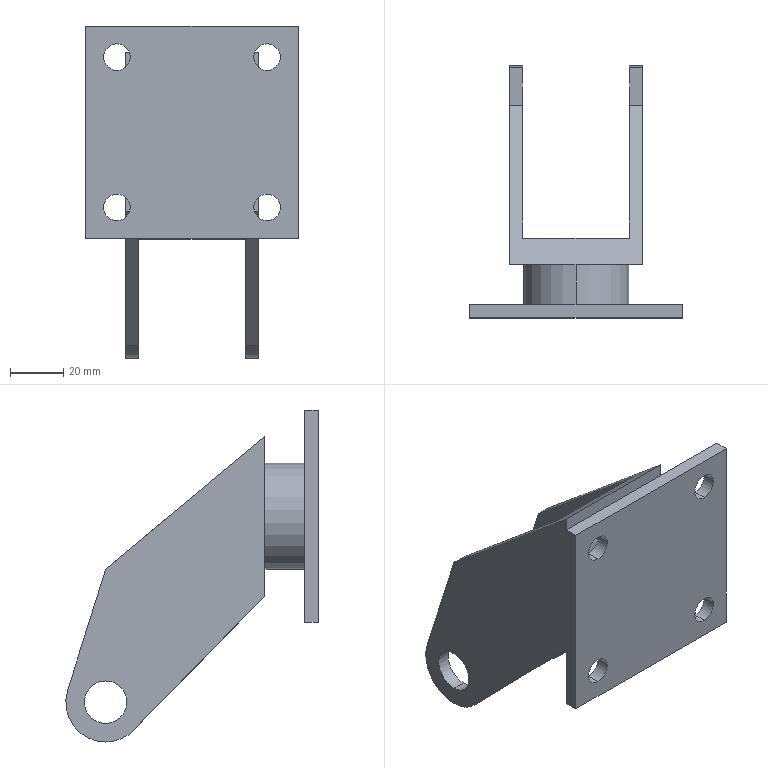Part | SolidWorks | features ICE 3, Extrusion 1 | 1 solid | 34 faces | box 80 x 95 x 125 mm | volume 116525 mm3 | cylinder 18 | plane 16 | commonest cylinder face diameters 10 x8 16 x4 30 x4 40 x2
STEP:
#1=CARTESIAN_POINT('',(0.,20.,20.));
#2=VERTEX_POINT('',#1);
#3=CARTESIAN_POINT('',(0.,20.,-20.));
#4=VERTEX_POINT('',#3);
#5=CARTESIAN_POINT('',(0.,20.,0.));
#6=DIRECTION('',(0.,1.,0.));
#7=DIRECTION('',(0.,0.,1.));
#8=AXIS2_PLACEMENT_3D('',#5,#6,#7);
#9=CIRCLE('',#8,20.);
#10=EDGE_CURVE('',#2,#4,#9,.T.);
#11=ORIENTED_EDGE('',*,*,#10,.F.);
#12=CARTESIAN_POINT('',(0.,5.,20.));
#13=VERTEX_POINT('',#12);
#14=CARTESIAN_POINT('',(0.,20.,20.));
#15=DIRECTION('',(0.,-1.,0.));
#16=VECTOR('',#15,1000.);
#17=LINE('',#14,#16);
#18=EDGE_CURVE('',#2,#13,#17,.T.);
#19=ORIENTED_EDGE('',*,*,#18,.T.);
#20=CARTESIAN_POINT('',(0.,5.,-20.));
#21=VERTEX_POINT('',#20);
#22=CARTESIAN_POINT('',(0.,5.,0.));
#23=DIRECTION('',(0.,1.,0.));
#24=DIRECTION('',(0.,0.,1.));
#25=AXIS2_PLACEMENT_3D('',#22,#23,#24);
#26=CIRCLE('',#25,20.);
#27=EDGE_CURVE('',#13,#21,#26,.T.);
#28=ORIENTED_EDGE('',*,*,#27,.T.);
#29=CARTESIAN_POINT('',(0.,20.,-20.));
#30=DIRECTION('',(0.,-1.,0.));
#31=VECTOR('',#30,1000.);
#32=LINE('',#29,#31);
#33=EDGE_CURVE('',#4,#21,#32,.T.);
#34=ORIENTED_EDGE('',*,*,#33,.F.);
#35=EDGE_LOOP('',(#11,#19,#28,#34));
#36=FACE_OUTER_BOUND('',#35,.T.);
#37=CARTESIAN_POINT('',(0.,20.,0.));
#38=DIRECTION('',(0.,-1.,0.));
#39=DIRECTION('',(0.,0.,-1.));
#40=AXIS2_PLACEMENT_3D('',#37,#38,#39);
#41=CYLINDRICAL_SURFACE('',#40,20.);
#42=ADVANCED_FACE('',(#36),#41,.T.);
#43=CARTESIAN_POINT('',(28.284,5.,23.284));
#44=VERTEX_POINT('',#43);
#45=CARTESIAN_POINT('',(28.284,5.,33.284));
#46=VERTEX_POINT('',#45);
#47=CARTESIAN_POINT('',(28.284,5.,28.284));
#48=DIRECTION('',(0.,1.,0.));
#49=DIRECTION('',(0.,0.,1.));
#50=AXIS2_PLACEMENT_3D('',#47,#48,#49);
#51=CIRCLE('',#50,5.);
#52=EDGE_CURVE('',#44,#46,#51,.T.);
#53=ORIENTED_EDGE('',*,*,#52,.T.);
#54=CARTESIAN_POINT('',(28.284,0.,33.284));
#55=VERTEX_POINT('',#54);
#56=CARTESIAN_POINT('',(28.284,5.,33.284));
#57=DIRECTION('',(0.,-1.,0.));
#58=VECTOR('',#57,1000.);
#59=LINE('',#56,#58);
#60=EDGE_CURVE('',#46,#55,#59,.T.);
#61=ORIENTED_EDGE('',*,*,#60,.T.);
#62=CARTESIAN_POINT('',(28.284,0.,23.284));
#63=VERTEX_POINT('',#62);
#64=CARTESIAN_POINT('',(28.284,0.,28.284));
#65=DIRECTION('',(0.,1.,0.));
#66=DIRECTION('',(0.,0.,1.));
#67=AXIS2_PLACEMENT_3D('',#64,#65,#66);
#68=CIRCLE('',#67,5.);
#69=EDGE_CURVE('',#63,#55,#68,.T.);
#70=ORIENTED_EDGE('',*,*,#69,.F.);
#71=CARTESIAN_POINT('',(28.284,5.,23.284));
#72=DIRECTION('',(0.,-1.,0.));
#73=VECTOR('',#72,1000.);
#74=LINE('',#71,#73);
#75=EDGE_CURVE('',#44,#63,#74,.T.);
#76=ORIENTED_EDGE('',*,*,#75,.F.);
#77=EDGE_LOOP('',(#53,#61,#70,#76));
#78=FACE_OUTER_BOUND('',#77,.T.);
#79=CARTESIAN_POINT('',(28.284,5.,28.284));
#80=DIRECTION('',(0.,-1.,0.));
#81=DIRECTION('',(0.,0.,-1.));
#82=AXIS2_PLACEMENT_3D('',#79,#80,#81);
#83=CYLINDRICAL_SURFACE('',#82,5.);
#84=ADVANCED_FACE('',(#78),#83,.F.);
#85=CARTESIAN_POINT('',(28.284,5.,-33.284));
#86=VERTEX_POINT('',#85);
#87=CARTESIAN_POINT('',(28.284,5.,-23.284));
#88=VERTEX_POINT('',#87);
#89=CARTESIAN_POINT('',(28.284,5.,-28.284));
#90=DIRECTION('',(0.,1.,0.));
#91=DIRECTION('',(0.,0.,1.));
#92=AXIS2_PLACEMENT_3D('',#89,#90,#91);
#93=CIRCLE('',#92,5.);
#94=EDGE_CURVE('',#86,#88,#93,.T.);
#95=ORIENTED_EDGE('',*,*,#94,.T.);
#96=CARTESIAN_POINT('',(28.284,0.,-23.284));
#97=VERTEX_POINT('',#96);
#98=CARTESIAN_POINT('',(28.284,5.,-23.284));
#99=DIRECTION('',(0.,-1.,0.));
#100=VECTOR('',#99,1000.);
#101=LINE('',#98,#100);
#102=EDGE_CURVE('',#88,#97,#101,.T.);
#103=ORIENTED_EDGE('',*,*,#102,.T.);
#104=CARTESIAN_POINT('',(28.284,0.,-33.284));
#105=VERTEX_POINT('',#104);
#106=CARTESIAN_POINT('',(28.284,0.,-28.284));
#107=DIRECTION('',(0.,1.,0.));
#108=DIRECTION('',(0.,0.,1.));
#109=AXIS2_PLACEMENT_3D('',#106,#107,#108);
#110=CIRCLE('',#109,5.);
#111=EDGE_CURVE('',#105,#97,#110,.T.);
#112=ORIENTED_EDGE('',*,*,#111,.F.);
#113=CARTESIAN_POINT('',(28.284,5.,-33.284));
#114=DIRECTION('',(0.,-1.,0.));
#115=VECTOR('',#114,1000.);
#116=LINE('',#113,#115);
#117=EDGE_CURVE('',#86,#105,#116,.T.);
#118=ORIENTED_EDGE('',*,*,#117,.F.);
#119=EDGE_LOOP('',(#95,#103,#112,#118));
#120=FACE_OUTER_BOUND('',#119,.T.);
#121=CARTESIAN_POINT('',(28.284,5.,-28.284));
#122=DIRECTION('',(0.,-1.,0.));
#123=DIRECTION('',(0.,0.,-1.));
#124=AXIS2_PLACEMENT_3D('',#121,#122,#123);
#125=CYLINDRICAL_SURFACE('',#124,5.);
#126=ADVANCED_FACE('',(#120),#125,.F.);
#127=CARTESIAN_POINT('',(-28.284,5.,-33.284));
#128=VERTEX_POINT('',#127);
#129=CARTESIAN_POINT('',(-28.284,5.,-23.284));
#130=VERTEX_POINT('',#129);
#131=CARTESIAN_POINT('',(-28.284,5.,-28.284));
#132=DIRECTION('',(0.,1.,0.));
#133=DIRECTION('',(0.,0.,1.));
#134=AXIS2_PLACEMENT_3D('',#131,#132,#133);
#135=CIRCLE('',#134,5.);
#136=EDGE_CURVE('',#128,#130,#135,.T.);
#137=ORIENTED_EDGE('',*,*,#136,.T.);
#138=CARTESIAN_POINT('',(-28.284,0.,-23.284));
#139=VERTEX_POINT('',#138);
#140=CARTESIAN_POINT('',(-28.284,5.,-23.284));
#141=DIRECTION('',(0.,-1.,0.));
#142=VECTOR('',#141,1000.);
#143=LINE('',#140,#142);
#144=EDGE_CURVE('',#130,#139,#143,.T.);
#145=ORIENTED_EDGE('',*,*,#144,.T.);
#146=CARTESIAN_POINT('',(-28.284,0.,-33.284));
#147=VERTEX_POINT('',#146);
#148=CARTESIAN_POINT('',(-28.284,0.,-28.284));
#149=DIRECTION('',(0.,1.,0.));
#150=DIRECTION('',(0.,0.,1.));
#151=AXIS2_PLACEMENT_3D('',#148,#149,#150);
#152=CIRCLE('',#151,5.);
#153=EDGE_CURVE('',#147,#139,#152,.T.);
#154=ORIENTED_EDGE('',*,*,#153,.F.);
#155=CARTESIAN_POINT('',(-28.284,5.,-33.284));
#156=DIRECTION('',(0.,-1.,0.));
#157=VECTOR('',#156,1000.);
#158=LINE('',#155,#157);
#159=EDGE_CURVE('',#128,#147,#158,.T.);
#160=ORIENTED_EDGE('',*,*,#159,.F.);
#161=EDGE_LOOP('',(#137,#145,#154,#160));
#162=FACE_OUTER_BOUND('',#161,.T.);
#163=CARTESIAN_POINT('',(-28.284,5.,-28.284));
#164=DIRECTION('',(0.,-1.,0.));
#165=DIRECTION('',(0.,0.,-1.));
#166=AXIS2_PLACEMENT_3D('',#163,#164,#165);
#167=CYLINDRICAL_SURFACE('',#166,5.);
#168=ADVANCED_FACE('',(#162),#167,.F.);
#169=CARTESIAN_POINT('',(-28.284,5.,23.284));
#170=VERTEX_POINT('',#169);
#171=CARTESIAN_POINT('',(-28.284,5.,33.284));
#172=VERTEX_POINT('',#171);
#173=CARTESIAN_POINT('',(-28.284,5.,28.284));
#174=DIRECTION('',(0.,1.,0.));
#175=DIRECTION('',(0.,0.,1.));
#176=AXIS2_PLACEMENT_3D('',#173,#174,#175);
#177=CIRCLE('',#176,5.);
#178=EDGE_CURVE('',#170,#172,#177,.T.);
#179=ORIENTED_EDGE('',*,*,#178,.T.);
#180=CARTESIAN_POINT('',(-28.284,0.,33.284));
#181=VERTEX_POINT('',#180);
#182=CARTESIAN_POINT('',(-28.284,5.,33.284));
#183=DIRECTION('',(0.,-1.,0.));
#184=VECTOR('',#183,1000.);
#185=LINE('',#182,#184);
#186=EDGE_CURVE('',#172,#181,#185,.T.);
#187=ORIENTED_EDGE('',*,*,#186,.T.);
#188=CARTESIAN_POINT('',(-28.284,0.,23.284));
#189=VERTEX_POINT('',#188);
#190=CARTESIAN_POINT('',(-28.284,0.,28.284));
#191=DIRECTION('',(0.,1.,0.));
#192=DIRECTION('',(0.,0.,1.));
#193=AXIS2_PLACEMENT_3D('',#190,#191,#192);
#194=CIRCLE('',#193,5.);
#195=EDGE_CURVE('',#189,#181,#194,.T.);
#196=ORIENTED_EDGE('',*,*,#195,.F.);
#197=CARTESIAN_POINT('',(-28.284,5.,23.284));
#198=DIRECTION('',(0.,-1.,0.));
#199=VECTOR('',#198,1000.);
#200=LINE('',#197,#199);
#201=EDGE_CURVE('',#170,#189,#200,.T.);
#202=ORIENTED_EDGE('',*,*,#201,.F.);
#203=EDGE_LOOP('',(#179,#187,#196,#202));
#204=FACE_OUTER_BOUND('',#203,.T.);
#205=CARTESIAN_POINT('',(-28.284,5.,28.284));
#206=DIRECTION('',(0.,-1.,0.));
#207=DIRECTION('',(0.,0.,-1.));
#208=AXIS2_PLACEMENT_3D('',#205,#206,#207);
#209=CYLINDRICAL_SURFACE('',#208,5.);
#210=ADVANCED_FACE('',(#204),#209,.F.);
#211=CARTESIAN_POINT('',(20.,80.,-62.));
#212=VERTEX_POINT('',#211);
#213=CARTESIAN_POINT('',(20.,80.,-78.));
#214=VERTEX_POINT('',#213);
#215=CARTESIAN_POINT('',(20.,80.,-70.));
#216=DIRECTION('',(1.,0.,0.));
#217=DIRECTION('',(0.,0.,1.));
#218=AXIS2_PLACEMENT_3D('',#215,#216,#217);
#219=CIRCLE('',#218,8.);
#220=EDGE_CURVE('',#212,#214,#219,.T.);
#221=ORIENTED_EDGE('',*,*,#220,.F.);
#222=CARTESIAN_POINT('',(25.,80.,-62.));
#223=VERTEX_POINT('',#222);
#224=CARTESIAN_POINT('',(-25.,80.,-62.));
#225=DIRECTION('',(1.,0.,0.));
#226=VECTOR('',#225,1000.);
#227=LINE('',#224,#226);
#228=EDGE_CURVE('',#212,#223,#227,.T.);
#229=ORIENTED_EDGE('',*,*,#228,.T.);
#230=CARTESIAN_POINT('',(25.,80.,-78.));
#231=VERTEX_POINT('',#230);
#232=CARTESIAN_POINT('',(25.,80.,-70.));
#233=DIRECTION('',(1.,0.,0.));
#234=DIRECTION('',(0.,0.,-1.));
#235=AXIS2_PLACEMENT_3D('',#232,#233,#234);
#236=CIRCLE('',#235,8.);
#237=EDGE_CURVE('',#223,#231,#236,.T.);
#238=ORIENTED_EDGE('',*,*,#237,.T.);
#239=CARTESIAN_POINT('',(-25.,80.,-78.));
#240=DIRECTION('',(1.,0.,0.));
#241=VECTOR('',#240,1000.);
#242=LINE('',#239,#241);
#243=EDGE_CURVE('',#214,#231,#242,.T.);
#244=ORIENTED_EDGE('',*,*,#243,.F.);
#245=EDGE_LOOP('',(#221,#229,#238,#244));
#246=FACE_OUTER_BOUND('',#245,.T.);
#247=CARTESIAN_POINT('',(-25.,80.,-70.));
#248=DIRECTION('',(1.,0.,0.));
#249=DIRECTION('',(0.,0.,-1.));
#250=AXIS2_PLACEMENT_3D('',#247,#248,#249);
#251=CYLINDRICAL_SURFACE('',#250,8.);
#252=ADVANCED_FACE('',(#246),#251,.F.);
#253=CARTESIAN_POINT('',(-25.,80.,-62.));
#254=VERTEX_POINT('',#253);
#255=CARTESIAN_POINT('',(-25.,80.,-78.));
#256=VERTEX_POINT('',#255);
#257=CARTESIAN_POINT('',(-25.,80.,-70.));
#258=DIRECTION('',(1.,0.,0.));
#259=DIRECTION('',(0.,0.,-1.));
#260=AXIS2_PLACEMENT_3D('',#257,#258,#259);
#261=CIRCLE('',#260,8.);
#262=EDGE_CURVE('',#254,#256,#261,.T.);
#263=ORIENTED_EDGE('',*,*,#262,.F.);
#264=CARTESIAN_POINT('',(-20.,80.,-62.));
#265=VERTEX_POINT('',#264);
#266=CARTESIAN_POINT('',(-25.,80.,-62.));
#267=DIRECTION('',(1.,0.,0.));
#268=VECTOR('',#267,1000.);
#269=LINE('',#266,#268);
#270=EDGE_CURVE('',#254,#265,#269,.T.);
#271=ORIENTED_EDGE('',*,*,#270,.T.);
#272=CARTESIAN_POINT('',(-20.,80.,-78.));
#273=VERTEX_POINT('',#272);
#274=CARTESIAN_POINT('',(-20.,80.,-70.));
#275=DIRECTION('',(-1.,0.,0.));
#276=DIRECTION('',(0.,0.,-1.));
#277=AXIS2_PLACEMENT_3D('',#274,#275,#276);
#278=CIRCLE('',#277,8.);
#279=EDGE_CURVE('',#273,#265,#278,.T.);
#280=ORIENTED_EDGE('',*,*,#279,.F.);
#281=CARTESIAN_POINT('',(-25.,80.,-78.));
#282=DIRECTION('',(1.,0.,0.));
#283=VECTOR('',#282,1000.);
#284=LINE('',#281,#283);
#285=EDGE_CURVE('',#256,#273,#284,.T.);
#286=ORIENTED_EDGE('',*,*,#285,.F.);
#287=EDGE_LOOP('',(#263,#271,#280,#286));
#288=FACE_OUTER_BOUND('',#287,.T.);
#289=CARTESIAN_POINT('',(-25.,80.,-70.));
#290=DIRECTION('',(1.,0.,0.));
#291=DIRECTION('',(0.,0.,-1.));
#292=AXIS2_PLACEMENT_3D('',#289,#290,#291);
#293=CYLINDRICAL_SURFACE('',#292,8.);
#294=ADVANCED_FACE('',(#288),#293,.F.);
#295=CARTESIAN_POINT('',(20.,69.265,-80.477));
#296=VERTEX_POINT('',#295);
#297=CARTESIAN_POINT('',(20.,80.,-85.));
#298=VERTEX_POINT('',#297);
#299=CARTESIAN_POINT('',(20.,80.,-70.));
#300=DIRECTION('',(1.,0.,0.));
#301=DIRECTION('',(0.,0.,1.));
#302=AXIS2_PLACEMENT_3D('',#299,#300,#301);
#303=CIRCLE('',#302,15.);
#304=EDGE_CURVE('',#296,#298,#303,.T.);
#305=ORIENTED_EDGE('',*,*,#304,.T.);
#306=CARTESIAN_POINT('',(25.,80.,-85.));
#307=VERTEX_POINT('',#306);
#308=CARTESIAN_POINT('',(-25.,80.,-85.));
#309=DIRECTION('',(1.,0.,0.));
#310=VECTOR('',#309,1000.);
#311=LINE('',#308,#310);
#312=EDGE_CURVE('',#298,#307,#311,.T.);
#313=ORIENTED_EDGE('',*,*,#312,.T.);
#314=CARTESIAN_POINT('',(25.,69.265,-80.477));
#315=VERTEX_POINT('',#314);
#316=CARTESIAN_POINT('',(25.,80.,-70.));
#317=DIRECTION('',(1.,0.,0.));
#318=DIRECTION('',(0.,0.,-1.));
#319=AXIS2_PLACEMENT_3D('',#316,#317,#318);
#320=CIRCLE('',#319,15.);
#321=EDGE_CURVE('',#315,#307,#320,.T.);
#322=ORIENTED_EDGE('',*,*,#321,.F.);
#323=CARTESIAN_POINT('',(-25.,69.265,-80.477));
#324=DIRECTION('',(1.,0.,0.));
#325=VECTOR('',#324,1000.);
#326=LINE('',#323,#325);
#327=EDGE_CURVE('',#296,#315,#326,.T.);
#328=ORIENTED_EDGE('',*,*,#327,.F.);
#329=EDGE_LOOP('',(#305,#313,#322,#328));
#330=FACE_OUTER_BOUND('',#329,.T.);
#331=CARTESIAN_POINT('',(-25.,80.,-70.));
#332=DIRECTION('',(1.,0.,0.));
#333=DIRECTION('',(0.,0.,-1.));
#334=AXIS2_PLACEMENT_3D('',#331,#332,#333);
#335=CYLINDRICAL_SURFACE('',#334,15.);
#336=ADVANCED_FACE('',(#330),#335,.T.);
#337=CARTESIAN_POINT('',(-25.,69.265,-80.477));
#338=VERTEX_POINT('',#337);
#339=CARTESIAN_POINT('',(-25.,80.,-85.));
#340=VERTEX_POINT('',#339);
#341=CARTESIAN_POINT('',(-25.,80.,-70.));
#342=DIRECTION('',(1.,0.,0.));
#343=DIRECTION('',(0.,0.,-1.));
#344=AXIS2_PLACEMENT_3D('',#341,#342,#343);
#345=CIRCLE('',#344,15.);
#346=EDGE_CURVE('',#338,#340,#345,.T.);
#347=ORIENTED_EDGE('',*,*,#346,.T.);
#348=CARTESIAN_POINT('',(-20.,80.,-85.));
#349=VERTEX_POINT('',#348);
#350=CARTESIAN_POINT('',(-25.,80.,-85.));
#351=DIRECTION('',(1.,0.,0.));
#352=VECTOR('',#351,1000.);
#353=LINE('',#350,#352);
#354=EDGE_CURVE('',#340,#349,#353,.T.);
#355=ORIENTED_EDGE('',*,*,#354,.T.);
#356=CARTESIAN_POINT('',(-20.,69.265,-80.477));
#357=VERTEX_POINT('',#356);
#358=CARTESIAN_POINT('',(-20.,80.,-70.));
#359=DIRECTION('',(-1.,0.,0.));
#360=DIRECTION('',(0.,0.,-1.));
#361=AXIS2_PLACEMENT_3D('',#358,#359,#360);
#362=CIRCLE('',#361,15.);
#363=EDGE_CURVE('',#349,#357,#362,.T.);
#364=ORIENTED_EDGE('',*,*,#363,.T.);
#365=CARTESIAN_POINT('',(-25.,69.265,-80.477));
#366=DIRECTION('',(1.,0.,0.));
#367=VECTOR('',#366,1000.);
#368=LINE('',#365,#367);
#369=EDGE_CURVE('',#338,#357,#368,.T.);
#370=ORIENTED_EDGE('',*,*,#369,.F.);
#371=EDGE_LOOP('',(#347,#355,#364,#370));
#372=FACE_OUTER_BOUND('',#371,.T.);
#373=CARTESIAN_POINT('',(-25.,80.,-70.));
#374=DIRECTION('',(1.,0.,0.));
#375=DIRECTION('',(0.,0.,-1.));
#376=AXIS2_PLACEMENT_3D('',#373,#374,#375);
#377=CYLINDRICAL_SURFACE('',#376,15.);
#378=ADVANCED_FACE('',(#372),#377,.T.);
#379=CARTESIAN_POINT('',(-20.,30.,21.667));
#380=VERTEX_POINT('',#379);
#381=CARTESIAN_POINT('',(20.,30.,21.667));
#382=VERTEX_POINT('',#381);
#383=CARTESIAN_POINT('',(-25.,30.,21.667));
#384=DIRECTION('',(1.,0.,0.));
#385=VECTOR('',#384,1000.);
#386=LINE('',#383,#385);
#387=EDGE_CURVE('',#380,#382,#386,.T.);
#388=ORIENTED_EDGE('',*,*,#387,.F.);
#389=CARTESIAN_POINT('',(-20.,80.,-20.));
#390=VERTEX_POINT('',#389);
#391=CARTESIAN_POINT('',(-20.,20.,30.));
#392=DIRECTION('',(0.,0.7682,-0.6402));
#393=VECTOR('',#392,1000.);
#394=LINE('',#391,#393);
#395=EDGE_CURVE('',#380,#390,#394,.T.);
#396=ORIENTED_EDGE('',*,*,#395,.T.);
#397=CARTESIAN_POINT('',(-25.,80.,-20.));
#398=VERTEX_POINT('',#397);
#399=CARTESIAN_POINT('',(-25.,80.,-20.));
#400=DIRECTION('',(1.,0.,0.));
#401=VECTOR('',#400,1000.);
#402=LINE('',#399,#401);
#403=EDGE_CURVE('',#398,#390,#402,.T.);
#404=ORIENTED_EDGE('',*,*,#403,.F.);
#405=CARTESIAN_POINT('',(-25.,20.,30.));
#406=VERTEX_POINT('',#405);
#407=CARTESIAN_POINT('',(-25.,20.,30.));
#408=DIRECTION('',(0.,-0.7682,0.6402));
#409=VECTOR('',#408,1000.);
#410=LINE('',#407,#409);
#411=EDGE_CURVE('',#398,#406,#410,.T.);
#412=ORIENTED_EDGE('',*,*,#411,.T.);
#413=CARTESIAN_POINT('',(25.,20.,30.));
#414=VERTEX_POINT('',#413);
#415=CARTESIAN_POINT('',(-25.,20.,30.));
#416=DIRECTION('',(1.,0.,0.));
#417=VECTOR('',#416,1000.);
#418=LINE('',#415,#417);
#419=EDGE_CURVE('',#406,#414,#418,.T.);
#420=ORIENTED_EDGE('',*,*,#419,.T.);
#421=CARTESIAN_POINT('',(25.,80.,-20.));
#422=VERTEX_POINT('',#421);
#423=CARTESIAN_POINT('',(25.,20.,30.));
#424=DIRECTION('',(0.,-0.7682,0.6402));
#425=VECTOR('',#424,1000.);
#426=LINE('',#423,#425);
#427=EDGE_CURVE('',#422,#414,#426,.T.);
#428=ORIENTED_EDGE('',*,*,#427,.F.);
#429=CARTESIAN_POINT('',(20.,80.,-20.));
#430=VERTEX_POINT('',#429);
#431=CARTESIAN_POINT('',(-25.,80.,-20.));
#432=DIRECTION('',(1.,0.,0.));
#433=VECTOR('',#432,1000.);
#434=LINE('',#431,#433);
#435=EDGE_CURVE('',#430,#422,#434,.T.);
#436=ORIENTED_EDGE('',*,*,#435,.F.);
#437=CARTESIAN_POINT('',(20.,20.,30.));
#438=DIRECTION('',(0.,-0.7682,0.6402));
#439=VECTOR('',#438,1000.);
#440=LINE('',#437,#439);
#441=EDGE_CURVE('',#430,#382,#440,.T.);
#442=ORIENTED_EDGE('',*,*,#441,.T.);
#443=EDGE_LOOP('',(#388,#396,#404,#412,#420,#428,#436,#442));
#444=FACE_OUTER_BOUND('',#443,.T.);
#445=CARTESIAN_POINT('',(-25.,20.,30.));
#446=DIRECTION('',(0.,0.6402,0.7682));
#447=DIRECTION('',(0.,-0.7682,0.6402));
#448=AXIS2_PLACEMENT_3D('',#445,#446,#447);
#449=PLANE('',#448);
#450=ADVANCED_FACE('',(#444),#449,.T.);
#451=ORIENTED_EDGE('',*,*,#403,.T.);
#452=CARTESIAN_POINT('',(-20.,94.309,-65.5));
#453=VERTEX_POINT('',#452);
#454=CARTESIAN_POINT('',(-20.,80.,-20.));
#455=DIRECTION('',(0.,0.3,-0.9539));
#456=VECTOR('',#455,1000.);
#457=LINE('',#454,#456);
#458=EDGE_CURVE('',#390,#453,#457,.T.);
#459=ORIENTED_EDGE('',*,*,#458,.T.);
#460=CARTESIAN_POINT('',(-25.,94.309,-65.5));
#461=VERTEX_POINT('',#460);
#462=CARTESIAN_POINT('',(-25.,94.309,-65.5));
#463=DIRECTION('',(1.,0.,0.));
#464=VECTOR('',#463,1000.);
#465=LINE('',#462,#464);
#466=EDGE_CURVE('',#461,#453,#465,.T.);
#467=ORIENTED_EDGE('',*,*,#466,.F.);
#468=CARTESIAN_POINT('',(-25.,80.,-20.));
#469=DIRECTION('',(0.,-0.3,0.9539));
#470=VECTOR('',#469,1000.);
#471=LINE('',#468,#470);
#472=EDGE_CURVE('',#461,#398,#471,.T.);
#473=ORIENTED_EDGE('',*,*,#472,.T.);
#474=EDGE_LOOP('',(#451,#459,#467,#473));
#475=FACE_OUTER_BOUND('',#474,.T.);
#476=CARTESIAN_POINT('',(-25.,80.,-20.));
#477=DIRECTION('',(0.,0.9539,0.3));
#478=DIRECTION('',(0.,-0.3,0.9539));
#479=AXIS2_PLACEMENT_3D('',#476,#477,#478);
#480=PLANE('',#479);
#481=ADVANCED_FACE('',(#475),#480,.T.);
#482=CARTESIAN_POINT('',(20.,94.309,-65.5));
#483=VERTEX_POINT('',#482);
#484=CARTESIAN_POINT('',(25.,94.309,-65.5));
#485=VERTEX_POINT('',#484);
#486=CARTESIAN_POINT('',(-25.,94.309,-65.5));
#487=DIRECTION('',(1.,0.,0.));
#488=VECTOR('',#487,1000.);
#489=LINE('',#486,#488);
#490=EDGE_CURVE('',#483,#485,#489,.T.);
#491=ORIENTED_EDGE('',*,*,#490,.F.);
#492=CARTESIAN_POINT('',(20.,80.,-20.));
#493=DIRECTION('',(0.,-0.3,0.9539));
#494=VECTOR('',#493,1000.);
#495=LINE('',#492,#494);
#496=EDGE_CURVE('',#483,#430,#495,.T.);
#497=ORIENTED_EDGE('',*,*,#496,.T.);
#498=ORIENTED_EDGE('',*,*,#435,.T.);
#499=CARTESIAN_POINT('',(25.,80.,-20.));
#500=DIRECTION('',(0.,-0.3,0.9539));
#501=VECTOR('',#500,1000.);
#502=LINE('',#499,#501);
#503=EDGE_CURVE('',#485,#422,#502,.T.);
#504=ORIENTED_EDGE('',*,*,#503,.F.);
#505=EDGE_LOOP('',(#491,#497,#498,#504));
#506=FACE_OUTER_BOUND('',#505,.T.);
#507=CARTESIAN_POINT('',(-25.,80.,-20.));
#508=DIRECTION('',(0.,0.9539,0.3));
#509=DIRECTION('',(0.,-0.3,0.9539));
#510=AXIS2_PLACEMENT_3D('',#507,#508,#509);
#511=PLANE('',#510);
#512=ADVANCED_FACE('',(#506),#511,.T.);
#513=ORIENTED_EDGE('',*,*,#354,.F.);
#514=CARTESIAN_POINT('',(-25.,80.,-70.));
#515=DIRECTION('',(1.,0.,0.));
#516=DIRECTION('',(0.,0.,-1.));
#517=AXIS2_PLACEMENT_3D('',#514,#515,#516);
#518=CIRCLE('',#517,15.);
#519=EDGE_CURVE('',#340,#461,#518,.T.);
#520=ORIENTED_EDGE('',*,*,#519,.T.);
#521=ORIENTED_EDGE('',*,*,#466,.T.);
#522=CARTESIAN_POINT('',(-20.,80.,-70.));
#523=DIRECTION('',(-1.,0.,0.));
#524=DIRECTION('',(0.,0.,-1.));
#525=AXIS2_PLACEMENT_3D('',#522,#523,#524);
#526=CIRCLE('',#525,15.);
#527=EDGE_CURVE('',#453,#349,#526,.T.);
#528=ORIENTED_EDGE('',*,*,#527,.T.);
#529=EDGE_LOOP('',(#513,#520,#521,#528));
#530=FACE_OUTER_BOUND('',#529,.T.);
#531=CARTESIAN_POINT('',(-25.,80.,-70.));
#532=DIRECTION('',(1.,0.,0.));
#533=DIRECTION('',(0.,0.,-1.));
#534=AXIS2_PLACEMENT_3D('',#531,#532,#533);
#535=CYLINDRICAL_SURFACE('',#534,15.);
#536=ADVANCED_FACE('',(#530),#535,.T.);
#537=ORIENTED_EDGE('',*,*,#312,.F.);
#538=CARTESIAN_POINT('',(20.,80.,-70.));
#539=DIRECTION('',(1.,0.,0.));
#540=DIRECTION('',(0.,0.,1.));
#541=AXIS2_PLACEMENT_3D('',#538,#539,#540);
#542=CIRCLE('',#541,15.);
#543=EDGE_CURVE('',#298,#483,#542,.T.);
#544=ORIENTED_EDGE('',*,*,#543,.T.);
#545=ORIENTED_EDGE('',*,*,#490,.T.);
#546=CARTESIAN_POINT('',(25.,80.,-70.));
#547=DIRECTION('',(1.,0.,0.));
#548=DIRECTION('',(0.,0.,-1.));
#549=AXIS2_PLACEMENT_3D('',#546,#547,#548);
#550=CIRCLE('',#549,15.);
#551=EDGE_CURVE('',#307,#485,#550,.T.);
#552=ORIENTED_EDGE('',*,*,#551,.F.);
#553=EDGE_LOOP('',(#537,#544,#545,#552));
#554=FACE_OUTER_BOUND('',#553,.T.);
#555=CARTESIAN_POINT('',(-25.,80.,-70.));
#556=DIRECTION('',(1.,0.,0.));
#557=DIRECTION('',(0.,0.,-1.));
#558=AXIS2_PLACEMENT_3D('',#555,#556,#557);
#559=CYLINDRICAL_SURFACE('',#558,15.);
#560=ADVANCED_FACE('',(#554),#559,.T.);
#561=ORIENTED_EDGE('',*,*,#369,.T.);
#562=CARTESIAN_POINT('',(-20.,30.,-40.246));
#563=VERTEX_POINT('',#562);
#564=CARTESIAN_POINT('',(-20.,20.,-30.));
#565=DIRECTION('',(0.,-0.6985,0.7156));
#566=VECTOR('',#565,1000.);
#567=LINE('',#564,#566);
#568=EDGE_CURVE('',#357,#563,#567,.T.);
#569=ORIENTED_EDGE('',*,*,#568,.T.);
#570=CARTESIAN_POINT('',(20.,30.,-40.246));
#571=VERTEX_POINT('',#570);
#572=CARTESIAN_POINT('',(-25.,30.,-40.246));
#573=DIRECTION('',(-1.,0.,0.));
#574=VECTOR('',#573,1000.);
#575=LINE('',#572,#574);
#576=EDGE_CURVE('',#571,#563,#575,.T.);
#577=ORIENTED_EDGE('',*,*,#576,.F.);
#578=CARTESIAN_POINT('',(20.,20.,-30.));
#579=DIRECTION('',(0.,0.6985,-0.7156));
#580=VECTOR('',#579,1000.);
#581=LINE('',#578,#580);
#582=EDGE_CURVE('',#571,#296,#581,.T.);
#583=ORIENTED_EDGE('',*,*,#582,.T.);
#584=ORIENTED_EDGE('',*,*,#327,.T.);
#585=CARTESIAN_POINT('',(25.,20.,-30.));
#586=VERTEX_POINT('',#585);
#587=CARTESIAN_POINT('',(25.,20.,-30.));
#588=DIRECTION('',(0.,0.6985,-0.7156));
#589=VECTOR('',#588,1000.);
#590=LINE('',#587,#589);
#591=EDGE_CURVE('',#586,#315,#590,.T.);
#592=ORIENTED_EDGE('',*,*,#591,.F.);
#593=CARTESIAN_POINT('',(-25.,20.,-30.));
#594=VERTEX_POINT('',#593);
#595=CARTESIAN_POINT('',(-25.,20.,-30.));
#596=DIRECTION('',(1.,0.,0.));
#597=VECTOR('',#596,1000.);
#598=LINE('',#595,#597);
#599=EDGE_CURVE('',#594,#586,#598,.T.);
#600=ORIENTED_EDGE('',*,*,#599,.F.);
#601=CARTESIAN_POINT('',(-25.,20.,-30.));
#602=DIRECTION('',(0.,0.6985,-0.7156));
#603=VECTOR('',#602,1000.);
#604=LINE('',#601,#603);
#605=EDGE_CURVE('',#594,#338,#604,.T.);
#606=ORIENTED_EDGE('',*,*,#605,.T.);
#607=EDGE_LOOP('',(#561,#569,#577,#583,#584,#592,#600,#606));
#608=FACE_OUTER_BOUND('',#607,.T.);
#609=CARTESIAN_POINT('',(-25.,20.,-30.));
#610=DIRECTION('',(0.,-0.7156,-0.6985));
#611=DIRECTION('',(0.,0.6985,-0.7156));
#612=AXIS2_PLACEMENT_3D('',#609,#610,#611);
#613=PLANE('',#612);
#614=ADVANCED_FACE('',(#608),#613,.T.);
#615=ORIENTED_EDGE('',*,*,#270,.F.);
#616=CARTESIAN_POINT('',(-25.,80.,-70.));
#617=DIRECTION('',(1.,0.,0.));
#618=DIRECTION('',(0.,0.,-1.));
#619=AXIS2_PLACEMENT_3D('',#616,#617,#618);
#620=CIRCLE('',#619,8.);
#621=EDGE_CURVE('',#256,#254,#620,.T.);
#622=ORIENTED_EDGE('',*,*,#621,.F.);
#623=ORIENTED_EDGE('',*,*,#285,.T.);
#624=CARTESIAN_POINT('',(-20.,80.,-70.));
#625=DIRECTION('',(-1.,0.,0.));
#626=DIRECTION('',(0.,0.,-1.));
#627=AXIS2_PLACEMENT_3D('',#624,#625,#626);
#628=CIRCLE('',#627,8.);
#629=EDGE_CURVE('',#265,#273,#628,.T.);
#630=ORIENTED_EDGE('',*,*,#629,.F.);
#631=EDGE_LOOP('',(#615,#622,#623,#630));
#632=FACE_OUTER_BOUND('',#631,.T.);
#633=CARTESIAN_POINT('',(-25.,80.,-70.));
#634=DIRECTION('',(1.,0.,0.));
#635=DIRECTION('',(0.,0.,-1.));
#636=AXIS2_PLACEMENT_3D('',#633,#634,#635);
#637=CYLINDRICAL_SURFACE('',#636,8.);
#638=ADVANCED_FACE('',(#632),#637,.F.);
#639=ORIENTED_EDGE('',*,*,#228,.F.);
#640=CARTESIAN_POINT('',(20.,80.,-70.));
#641=DIRECTION('',(1.,0.,0.));
#642=DIRECTION('',(0.,0.,1.));
#643=AXIS2_PLACEMENT_3D('',#640,#641,#642);
#644=CIRCLE('',#643,8.);
#645=EDGE_CURVE('',#214,#212,#644,.T.);
#646=ORIENTED_EDGE('',*,*,#645,.F.);
#647=ORIENTED_EDGE('',*,*,#243,.T.);
#648=CARTESIAN_POINT('',(25.,80.,-70.));
#649=DIRECTION('',(1.,0.,0.));
#650=DIRECTION('',(0.,0.,-1.));
#651=AXIS2_PLACEMENT_3D('',#648,#649,#650);
#652=CIRCLE('',#651,8.);
#653=EDGE_CURVE('',#231,#223,#652,.T.);
#654=ORIENTED_EDGE('',*,*,#653,.T.);
#655=EDGE_LOOP('',(#639,#646,#647,#654));
#656=FACE_OUTER_BOUND('',#655,.T.);
#657=CARTESIAN_POINT('',(-25.,80.,-70.));
#658=DIRECTION('',(1.,0.,0.));
#659=DIRECTION('',(0.,0.,-1.));
#660=AXIS2_PLACEMENT_3D('',#657,#658,#659);
#661=CYLINDRICAL_SURFACE('',#660,8.);
#662=ADVANCED_FACE('',(#656),#661,.F.);
#663=CARTESIAN_POINT('',(0.,5.,0.));
#664=DIRECTION('',(0.,1.,0.));
#665=DIRECTION('',(0.,0.,1.));
#666=AXIS2_PLACEMENT_3D('',#663,#664,#665);
#667=CIRCLE('',#666,20.);
#668=EDGE_CURVE('',#21,#13,#667,.T.);
#669=ORIENTED_EDGE('',*,*,#668,.F.);
#670=ORIENTED_EDGE('',*,*,#27,.F.);
#671=EDGE_LOOP('',(#669,#670));
#672=FACE_BOUND('',#671,.T.);
#673=ORIENTED_EDGE('',*,*,#94,.F.);
#674=CARTESIAN_POINT('',(28.284,5.,-28.284));
#675=DIRECTION('',(0.,1.,0.));
#676=DIRECTION('',(0.,0.,1.));
#677=AXIS2_PLACEMENT_3D('',#674,#675,#676);
#678=CIRCLE('',#677,5.);
#679=EDGE_CURVE('',#88,#86,#678,.T.);
#680=ORIENTED_EDGE('',*,*,#679,.F.);
#681=EDGE_LOOP('',(#673,#680));
#682=FACE_BOUND('',#681,.T.);
#683=ORIENTED_EDGE('',*,*,#178,.F.);
#684=CARTESIAN_POINT('',(-28.284,5.,28.284));
#685=DIRECTION('',(0.,1.,0.));
#686=DIRECTION('',(0.,0.,1.));
#687=AXIS2_PLACEMENT_3D('',#684,#685,#686);
#688=CIRCLE('',#687,5.);
#689=EDGE_CURVE('',#172,#170,#688,.T.);
#690=ORIENTED_EDGE('',*,*,#689,.F.);
#691=EDGE_LOOP('',(#683,#690));
#692=FACE_BOUND('',#691,.T.);
#693=CARTESIAN_POINT('',(40.,5.,40.));
#694=VERTEX_POINT('',#693);
#695=CARTESIAN_POINT('',(40.,5.,-40.));
#696=VERTEX_POINT('',#695);
#697=CARTESIAN_POINT('',(40.,5.,-40.));
#698=DIRECTION('',(0.,0.,-1.));
#699=VECTOR('',#698,1000.);
#700=LINE('',#697,#699);
#701=EDGE_CURVE('',#694,#696,#700,.T.);
#702=ORIENTED_EDGE('',*,*,#701,.T.);
#703=CARTESIAN_POINT('',(-40.,5.,-40.));
#704=VERTEX_POINT('',#703);
#705=CARTESIAN_POINT('',(-40.,5.,-40.));
#706=DIRECTION('',(-1.,0.,0.));
#707=VECTOR('',#706,1000.);
#708=LINE('',#705,#707);
#709=EDGE_CURVE('',#696,#704,#708,.T.);
#710=ORIENTED_EDGE('',*,*,#709,.T.);
#711=CARTESIAN_POINT('',(-40.,5.,40.));
#712=VERTEX_POINT('',#711);
#713=CARTESIAN_POINT('',(-40.,5.,-40.));
#714=DIRECTION('',(0.,0.,1.));
#715=VECTOR('',#714,1000.);
#716=LINE('',#713,#715);
#717=EDGE_CURVE('',#704,#712,#716,.T.);
#718=ORIENTED_EDGE('',*,*,#717,.T.);
#719=CARTESIAN_POINT('',(-40.,5.,40.));
#720=DIRECTION('',(1.,0.,0.));
#721=VECTOR('',#720,1000.);
#722=LINE('',#719,#721);
#723=EDGE_CURVE('',#712,#694,#722,.T.);
#724=ORIENTED_EDGE('',*,*,#723,.T.);
#725=EDGE_LOOP('',(#702,#710,#718,#724));
#726=FACE_OUTER_BOUND('',#725,.T.);
#727=ORIENTED_EDGE('',*,*,#136,.F.);
#728=CARTESIAN_POINT('',(-28.284,5.,-28.284));
#729=DIRECTION('',(0.,1.,0.));
#730=DIRECTION('',(0.,0.,1.));
#731=AXIS2_PLACEMENT_3D('',#728,#729,#730);
#732=CIRCLE('',#731,5.);
#733=EDGE_CURVE('',#130,#128,#732,.T.);
#734=ORIENTED_EDGE('',*,*,#733,.F.);
#735=EDGE_LOOP('',(#727,#734));
#736=FACE_BOUND('',#735,.T.);
#737=ORIENTED_EDGE('',*,*,#52,.F.);
#738=CARTESIAN_POINT('',(28.284,5.,28.284));
#739=DIRECTION('',(0.,1.,0.));
#740=DIRECTION('',(0.,0.,1.));
#741=AXIS2_PLACEMENT_3D('',#738,#739,#740);
#742=CIRCLE('',#741,5.);
#743=EDGE_CURVE('',#46,#44,#742,.T.);
#744=ORIENTED_EDGE('',*,*,#743,.F.);
#745=EDGE_LOOP('',(#737,#744));
#746=FACE_BOUND('',#745,.T.);
#747=CARTESIAN_POINT('',(0.,5.,0.));
#748=DIRECTION('',(0.,1.,0.));
#749=DIRECTION('',(0.,0.,1.));
#750=AXIS2_PLACEMENT_3D('',#747,#748,#749);
#751=PLANE('',#750);
#752=ADVANCED_FACE('',(#672,#682,#692,#726,#736,#746),#751,.T.);
#753=CARTESIAN_POINT('',(40.,0.,40.));
#754=VERTEX_POINT('',#753);
#755=CARTESIAN_POINT('',(40.,0.,-40.));
#756=VERTEX_POINT('',#755);
#757=CARTESIAN_POINT('',(40.,0.,-40.));
#758=DIRECTION('',(0.,0.,-1.));
#759=VECTOR('',#758,1000.);
#760=LINE('',#757,#759);
#761=EDGE_CURVE('',#754,#756,#760,.T.);
#762=ORIENTED_EDGE('',*,*,#761,.F.);
#763=CARTESIAN_POINT('',(-40.,0.,40.));
#764=VERTEX_POINT('',#763);
#765=CARTESIAN_POINT('',(-40.,0.,40.));
#766=DIRECTION('',(1.,0.,0.));
#767=VECTOR('',#766,1000.);
#768=LINE('',#765,#767);
#769=EDGE_CURVE('',#764,#754,#768,.T.);
#770=ORIENTED_EDGE('',*,*,#769,.F.);
#771=CARTESIAN_POINT('',(-40.,0.,-40.));
#772=VERTEX_POINT('',#771);
#773=CARTESIAN_POINT('',(-40.,0.,-40.));
#774=DIRECTION('',(0.,0.,1.));
#775=VECTOR('',#774,1000.);
#776=LINE('',#773,#775);
#777=EDGE_CURVE('',#772,#764,#776,.T.);
#778=ORIENTED_EDGE('',*,*,#777,.F.);
#779=CARTESIAN_POINT('',(-40.,0.,-40.));
#780=DIRECTION('',(-1.,0.,0.));
#781=VECTOR('',#780,1000.);
#782=LINE('',#779,#781);
#783=EDGE_CURVE('',#756,#772,#782,.T.);
#784=ORIENTED_EDGE('',*,*,#783,.F.);
#785=EDGE_LOOP('',(#762,#770,#778,#784));
#786=FACE_OUTER_BOUND('',#785,.T.);
#787=ORIENTED_EDGE('',*,*,#195,.T.);
#788=CARTESIAN_POINT('',(-28.284,0.,28.284));
#789=DIRECTION('',(0.,1.,0.));
#790=DIRECTION('',(0.,0.,1.));
#791=AXIS2_PLACEMENT_3D('',#788,#789,#790);
#792=CIRCLE('',#791,5.);
#793=EDGE_CURVE('',#181,#189,#792,.T.);
#794=ORIENTED_EDGE('',*,*,#793,.T.);
#795=EDGE_LOOP('',(#787,#794));
#796=FACE_BOUND('',#795,.T.);
#797=ORIENTED_EDGE('',*,*,#153,.T.);
#798=CARTESIAN_POINT('',(-28.284,0.,-28.284));
#799=DIRECTION('',(0.,1.,0.));
#800=DIRECTION('',(0.,0.,1.));
#801=AXIS2_PLACEMENT_3D('',#798,#799,#800);
#802=CIRCLE('',#801,5.);
#803=EDGE_CURVE('',#139,#147,#802,.T.);
#804=ORIENTED_EDGE('',*,*,#803,.T.);
#805=EDGE_LOOP('',(#797,#804));
#806=FACE_BOUND('',#805,.T.);
#807=ORIENTED_EDGE('',*,*,#111,.T.);
#808=CARTESIAN_POINT('',(28.284,0.,-28.284));
#809=DIRECTION('',(0.,1.,0.));
#810=DIRECTION('',(0.,0.,1.));
#811=AXIS2_PLACEMENT_3D('',#808,#809,#810);
#812=CIRCLE('',#811,5.);
#813=EDGE_CURVE('',#97,#105,#812,.T.);
#814=ORIENTED_EDGE('',*,*,#813,.T.);
#815=EDGE_LOOP('',(#807,#814));
#816=FACE_BOUND('',#815,.T.);
#817=ORIENTED_EDGE('',*,*,#69,.T.);
#818=CARTESIAN_POINT('',(28.284,0.,28.284));
#819=DIRECTION('',(0.,1.,0.));
#820=DIRECTION('',(0.,0.,1.));
#821=AXIS2_PLACEMENT_3D('',#818,#819,#820);
#822=CIRCLE('',#821,5.);
#823=EDGE_CURVE('',#55,#63,#822,.T.);
#824=ORIENTED_EDGE('',*,*,#823,.T.);
#825=EDGE_LOOP('',(#817,#824));
#826=FACE_BOUND('',#825,.T.);
#827=CARTESIAN_POINT('',(0.,0.,0.));
#828=DIRECTION('',(0.,1.,0.));
#829=DIRECTION('',(0.,0.,1.));
#830=AXIS2_PLACEMENT_3D('',#827,#828,#829);
#831=PLANE('',#830);
#832=ADVANCED_FACE('',(#786,#796,#806,#816,#826),#831,.F.);
#833=ORIENTED_EDGE('',*,*,#761,.T.);
#834=CARTESIAN_POINT('',(40.,5.,-40.));
#835=DIRECTION('',(0.,-1.,0.));
#836=VECTOR('',#835,1000.);
#837=LINE('',#834,#836);
#838=EDGE_CURVE('',#696,#756,#837,.T.);
#839=ORIENTED_EDGE('',*,*,#838,.F.);
#840=ORIENTED_EDGE('',*,*,#701,.F.);
#841=CARTESIAN_POINT('',(40.,5.,40.));
#842=DIRECTION('',(0.,-1.,0.));
#843=VECTOR('',#842,1000.);
#844=LINE('',#841,#843);
#845=EDGE_CURVE('',#694,#754,#844,.T.);
#846=ORIENTED_EDGE('',*,*,#845,.T.);
#847=EDGE_LOOP('',(#833,#839,#840,#846));
#848=FACE_OUTER_BOUND('',#847,.T.);
#849=CARTESIAN_POINT('',(40.,5.,-40.));
#850=DIRECTION('',(-1.,0.,0.));
#851=DIRECTION('',(0.,0.,1.));
#852=AXIS2_PLACEMENT_3D('',#849,#850,#851);
#853=PLANE('',#852);
#854=ADVANCED_FACE('',(#848),#853,.F.);
#855=ORIENTED_EDGE('',*,*,#783,.T.);
#856=CARTESIAN_POINT('',(-40.,5.,-40.));
#857=DIRECTION('',(0.,-1.,0.));
#858=VECTOR('',#857,1000.);
#859=LINE('',#856,#858);
#860=EDGE_CURVE('',#704,#772,#859,.T.);
#861=ORIENTED_EDGE('',*,*,#860,.F.);
#862=ORIENTED_EDGE('',*,*,#709,.F.);
#863=ORIENTED_EDGE('',*,*,#838,.T.);
#864=EDGE_LOOP('',(#855,#861,#862,#863));
#865=FACE_OUTER_BOUND('',#864,.T.);
#866=CARTESIAN_POINT('',(-40.,5.,-40.));
#867=DIRECTION('',(0.,0.,1.));
#868=DIRECTION('',(1.,0.,0.));
#869=AXIS2_PLACEMENT_3D('',#866,#867,#868);
#870=PLANE('',#869);
#871=ADVANCED_FACE('',(#865),#870,.F.);
#872=ORIENTED_EDGE('',*,*,#777,.T.);
#873=CARTESIAN_POINT('',(-40.,5.,40.));
#874=DIRECTION('',(0.,-1.,0.));
#875=VECTOR('',#874,1000.);
#876=LINE('',#873,#875);
#877=EDGE_CURVE('',#712,#764,#876,.T.);
#878=ORIENTED_EDGE('',*,*,#877,.F.);
#879=ORIENTED_EDGE('',*,*,#717,.F.);
#880=ORIENTED_EDGE('',*,*,#860,.T.);
#881=EDGE_LOOP('',(#872,#878,#879,#880));
#882=FACE_OUTER_BOUND('',#881,.T.);
#883=CARTESIAN_POINT('',(-40.,5.,-40.));
#884=DIRECTION('',(1.,0.,0.));
#885=DIRECTION('',(0.,0.,-1.));
#886=AXIS2_PLACEMENT_3D('',#883,#884,#885);
#887=PLANE('',#886);
#888=ADVANCED_FACE('',(#882),#887,.F.);
#889=ORIENTED_EDGE('',*,*,#769,.T.);
#890=ORIENTED_EDGE('',*,*,#845,.F.);
#891=ORIENTED_EDGE('',*,*,#723,.F.);
#892=ORIENTED_EDGE('',*,*,#877,.T.);
#893=EDGE_LOOP('',(#889,#890,#891,#892));
#894=FACE_OUTER_BOUND('',#893,.T.);
#895=CARTESIAN_POINT('',(-40.,5.,40.));
#896=DIRECTION('',(0.,0.,-1.));
#897=DIRECTION('',(-1.,0.,0.));
#898=AXIS2_PLACEMENT_3D('',#895,#896,#897);
#899=PLANE('',#898);
#900=ADVANCED_FACE('',(#894),#899,.F.);
#901=ORIENTED_EDGE('',*,*,#186,.F.);
#902=ORIENTED_EDGE('',*,*,#689,.T.);
#903=ORIENTED_EDGE('',*,*,#201,.T.);
#904=ORIENTED_EDGE('',*,*,#793,.F.);
#905=EDGE_LOOP('',(#901,#902,#903,#904));
#906=FACE_OUTER_BOUND('',#905,.T.);
#907=CARTESIAN_POINT('',(-28.284,5.,28.284));
#908=DIRECTION('',(0.,-1.,0.));
#909=DIRECTION('',(0.,0.,-1.));
#910=AXIS2_PLACEMENT_3D('',#907,#908,#909);
#911=CYLINDRICAL_SURFACE('',#910,5.);
#912=ADVANCED_FACE('',(#906),#911,.F.);
#913=ORIENTED_EDGE('',*,*,#144,.F.);
#914=ORIENTED_EDGE('',*,*,#733,.T.);
#915=ORIENTED_EDGE('',*,*,#159,.T.);
#916=ORIENTED_EDGE('',*,*,#803,.F.);
#917=EDGE_LOOP('',(#913,#914,#915,#916));
#918=FACE_OUTER_BOUND('',#917,.T.);
#919=CARTESIAN_POINT('',(-28.284,5.,-28.284));
#920=DIRECTION('',(0.,-1.,0.));
#921=DIRECTION('',(0.,0.,-1.));
#922=AXIS2_PLACEMENT_3D('',#919,#920,#921);
#923=CYLINDRICAL_SURFACE('',#922,5.);
#924=ADVANCED_FACE('',(#918),#923,.F.);
#925=ORIENTED_EDGE('',*,*,#102,.F.);
#926=ORIENTED_EDGE('',*,*,#679,.T.);
#927=ORIENTED_EDGE('',*,*,#117,.T.);
#928=ORIENTED_EDGE('',*,*,#813,.F.);
#929=EDGE_LOOP('',(#925,#926,#927,#928));
#930=FACE_OUTER_BOUND('',#929,.T.);
#931=CARTESIAN_POINT('',(28.284,5.,-28.284));
#932=DIRECTION('',(0.,-1.,0.));
#933=DIRECTION('',(0.,0.,-1.));
#934=AXIS2_PLACEMENT_3D('',#931,#932,#933);
#935=CYLINDRICAL_SURFACE('',#934,5.);
#936=ADVANCED_FACE('',(#930),#935,.F.);
#937=ORIENTED_EDGE('',*,*,#60,.F.);
#938=ORIENTED_EDGE('',*,*,#743,.T.);
#939=ORIENTED_EDGE('',*,*,#75,.T.);
#940=ORIENTED_EDGE('',*,*,#823,.F.);
#941=EDGE_LOOP('',(#937,#938,#939,#940));
#942=FACE_OUTER_BOUND('',#941,.T.);
#943=CARTESIAN_POINT('',(28.284,5.,28.284));
#944=DIRECTION('',(0.,-1.,0.));
#945=DIRECTION('',(0.,0.,-1.));
#946=AXIS2_PLACEMENT_3D('',#943,#944,#945);
#947=CYLINDRICAL_SURFACE('',#946,5.);
#948=ADVANCED_FACE('',(#942),#947,.F.);
#949=ORIENTED_EDGE('',*,*,#18,.F.);
#950=CARTESIAN_POINT('',(0.,20.,0.));
#951=DIRECTION('',(0.,1.,0.));
#952=DIRECTION('',(0.,0.,1.));
#953=AXIS2_PLACEMENT_3D('',#950,#951,#952);
#954=CIRCLE('',#953,20.);
#955=EDGE_CURVE('',#4,#2,#954,.T.);
#956=ORIENTED_EDGE('',*,*,#955,.F.);
#957=ORIENTED_EDGE('',*,*,#33,.T.);
#958=ORIENTED_EDGE('',*,*,#668,.T.);
#959=EDGE_LOOP('',(#949,#956,#957,#958));
#960=FACE_OUTER_BOUND('',#959,.T.);
#961=CARTESIAN_POINT('',(0.,20.,0.));
#962=DIRECTION('',(0.,-1.,0.));
#963=DIRECTION('',(0.,0.,-1.));
#964=AXIS2_PLACEMENT_3D('',#961,#962,#963);
#965=CYLINDRICAL_SURFACE('',#964,20.);
#966=ADVANCED_FACE('',(#960),#965,.T.);
#967=ORIENTED_EDGE('',*,*,#955,.T.);
#968=ORIENTED_EDGE('',*,*,#10,.T.);
#969=EDGE_LOOP('',(#967,#968));
#970=FACE_BOUND('',#969,.T.);
#971=ORIENTED_EDGE('',*,*,#599,.T.);
#972=CARTESIAN_POINT('',(25.,20.,0.));
#973=DIRECTION('',(0.,0.,-1.));
#974=VECTOR('',#973,1000.);
#975=LINE('',#972,#974);
#976=EDGE_CURVE('',#414,#586,#975,.T.);
#977=ORIENTED_EDGE('',*,*,#976,.F.);
#978=ORIENTED_EDGE('',*,*,#419,.F.);
#979=CARTESIAN_POINT('',(-25.,20.,0.));
#980=DIRECTION('',(0.,0.,-1.));
#981=VECTOR('',#980,1000.);
#982=LINE('',#979,#981);
#983=EDGE_CURVE('',#406,#594,#982,.T.);
#984=ORIENTED_EDGE('',*,*,#983,.T.);
#985=EDGE_LOOP('',(#971,#977,#978,#984));
#986=FACE_OUTER_BOUND('',#985,.T.);
#987=CARTESIAN_POINT('',(-25.,20.,0.));
#988=DIRECTION('',(0.,-1.,0.));
#989=DIRECTION('',(0.,0.,-1.));
#990=AXIS2_PLACEMENT_3D('',#987,#988,#989);
#991=PLANE('',#990);
#992=ADVANCED_FACE('',(#970,#986),#991,.T.);
#993=ORIENTED_EDGE('',*,*,#621,.T.);
#994=ORIENTED_EDGE('',*,*,#262,.T.);
#995=EDGE_LOOP('',(#993,#994));
#996=FACE_BOUND('',#995,.T.);
#997=ORIENTED_EDGE('',*,*,#983,.F.);
#998=ORIENTED_EDGE('',*,*,#411,.F.);
#999=ORIENTED_EDGE('',*,*,#472,.F.);
#1000=ORIENTED_EDGE('',*,*,#519,.F.);
#1001=ORIENTED_EDGE('',*,*,#346,.F.);
#1002=ORIENTED_EDGE('',*,*,#605,.F.);
#1003=EDGE_LOOP('',(#997,#998,#999,#1000,#1001,#1002));
#1004=FACE_OUTER_BOUND('',#1003,.T.);
#1005=CARTESIAN_POINT('',(-25.,80.,-70.));
#1006=DIRECTION('',(1.,0.,0.));
#1007=DIRECTION('',(0.,0.,-1.));
#1008=AXIS2_PLACEMENT_3D('',#1005,#1006,#1007);
#1009=PLANE('',#1008);
#1010=ADVANCED_FACE('',(#996,#1004),#1009,.F.);
#1011=ORIENTED_EDGE('',*,*,#976,.T.);
#1012=ORIENTED_EDGE('',*,*,#591,.T.);
#1013=ORIENTED_EDGE('',*,*,#321,.T.);
#1014=ORIENTED_EDGE('',*,*,#551,.T.);
#1015=ORIENTED_EDGE('',*,*,#503,.T.);
#1016=ORIENTED_EDGE('',*,*,#427,.T.);
#1017=EDGE_LOOP('',(#1011,#1012,#1013,#1014,#1015,#1016));
#1018=FACE_OUTER_BOUND('',#1017,.T.);
#1019=ORIENTED_EDGE('',*,*,#653,.F.);
#1020=ORIENTED_EDGE('',*,*,#237,.F.);
#1021=EDGE_LOOP('',(#1019,#1020));
#1022=FACE_BOUND('',#1021,.T.);
#1023=CARTESIAN_POINT('',(25.,80.,-70.));
#1024=DIRECTION('',(1.,0.,0.));
#1025=DIRECTION('',(0.,0.,-1.));
#1026=AXIS2_PLACEMENT_3D('',#1023,#1024,#1025);
#1027=PLANE('',#1026);
#1028=ADVANCED_FACE('',(#1018,#1022),#1027,.T.);
#1029=CARTESIAN_POINT('',(-20.,30.,-100.));
#1030=DIRECTION('',(0.,0.,-1.));
#1031=VECTOR('',#1030,1000.);
#1032=LINE('',#1029,#1031);
#1033=EDGE_CURVE('',#380,#563,#1032,.T.);
#1034=ORIENTED_EDGE('',*,*,#1033,.T.);
#1035=ORIENTED_EDGE('',*,*,#568,.F.);
#1036=ORIENTED_EDGE('',*,*,#363,.F.);
#1037=ORIENTED_EDGE('',*,*,#527,.F.);
#1038=ORIENTED_EDGE('',*,*,#458,.F.);
#1039=ORIENTED_EDGE('',*,*,#395,.F.);
#1040=EDGE_LOOP('',(#1034,#1035,#1036,#1037,#1038,#1039));
#1041=FACE_OUTER_BOUND('',#1040,.T.);
#1042=ORIENTED_EDGE('',*,*,#279,.T.);
#1043=ORIENTED_EDGE('',*,*,#629,.T.);
#1044=EDGE_LOOP('',(#1042,#1043));
#1045=FACE_BOUND('',#1044,.T.);
#1046=CARTESIAN_POINT('',(-20.,30.,-100.));
#1047=DIRECTION('',(1.,0.,0.));
#1048=DIRECTION('',(0.,0.,-1.));
#1049=AXIS2_PLACEMENT_3D('',#1046,#1047,#1048);
#1050=PLANE('',#1049);
#1051=ADVANCED_FACE('',(#1041,#1045),#1050,.T.);
#1052=ORIENTED_EDGE('',*,*,#496,.F.);
#1053=ORIENTED_EDGE('',*,*,#543,.F.);
#1054=ORIENTED_EDGE('',*,*,#304,.F.);
#1055=ORIENTED_EDGE('',*,*,#582,.F.);
#1056=CARTESIAN_POINT('',(20.,30.,-100.));
#1057=DIRECTION('',(0.,0.,1.));
#1058=VECTOR('',#1057,1000.);
#1059=LINE('',#1056,#1058);
#1060=EDGE_CURVE('',#571,#382,#1059,.T.);
#1061=ORIENTED_EDGE('',*,*,#1060,.T.);
#1062=ORIENTED_EDGE('',*,*,#441,.F.);
#1063=EDGE_LOOP('',(#1052,#1053,#1054,#1055,#1061,#1062));
#1064=FACE_OUTER_BOUND('',#1063,.T.);
#1065=ORIENTED_EDGE('',*,*,#645,.T.);
#1066=ORIENTED_EDGE('',*,*,#220,.T.);
#1067=EDGE_LOOP('',(#1065,#1066));
#1068=FACE_BOUND('',#1067,.T.);
#1069=CARTESIAN_POINT('',(20.,30.,-100.));
#1070=DIRECTION('',(-1.,0.,0.));
#1071=DIRECTION('',(0.,0.,1.));
#1072=AXIS2_PLACEMENT_3D('',#1069,#1070,#1071);
#1073=PLANE('',#1072);
#1074=ADVANCED_FACE('',(#1064,#1068),#1073,.T.);
#1075=ORIENTED_EDGE('',*,*,#387,.T.);
#1076=ORIENTED_EDGE('',*,*,#1060,.F.);
#1077=ORIENTED_EDGE('',*,*,#576,.T.);
#1078=ORIENTED_EDGE('',*,*,#1033,.F.);
#1079=EDGE_LOOP('',(#1075,#1076,#1077,#1078));
#1080=FACE_OUTER_BOUND('',#1079,.T.);
#1081=CARTESIAN_POINT('',(0.,30.,0.));
#1082=DIRECTION('',(0.,-1.,0.));
#1083=DIRECTION('',(0.,0.,-1.));
#1084=AXIS2_PLACEMENT_3D('',#1081,#1082,#1083);
#1085=PLANE('',#1084);
#1086=ADVANCED_FACE('',(#1080),#1085,.F.);
#1087=CLOSED_SHELL('',(#42,#84,#126,#168,#210,#252,#294,#336,#378,#450,#481,#512,#536,#560,#614,#638,#662,#752,#832,#854,#871,#888,#900,#912,#924,#936,#948,#966,#992,#1010,#1028,#1051,#1074,#1086));
#1088=MANIFOLD_SOLID_BREP('',#1087);
#1089=CARTESIAN_POINT('',(0.,0.,0.));
#1090=DIRECTION('',(0.,0.,1.));
#1091=DIRECTION('',(1.,0.,0.));
#1092=AXIS2_PLACEMENT_3D('',#1089,#1090,#1091);
#1093=(LENGTH_UNIT()NAMED_UNIT(*)SI_UNIT(.MILLI.,.METRE.));
#1094=UNCERTAINTY_MEASURE_WITH_UNIT(LENGTH_MEASURE(0.00001),#1093,'','');
#1095=(NAMED_UNIT(*)PLANE_ANGLE_UNIT()SI_UNIT($,.RADIAN.));
#1096=(NAMED_UNIT(*)SI_UNIT($,.STERADIAN.)SOLID_ANGLE_UNIT());
#1097=(GEOMETRIC_REPRESENTATION_CONTEXT(3)GLOBAL_UNCERTAINTY_ASSIGNED_CONTEXT((#1094))GLOBAL_UNIT_ASSIGNED_CONTEXT((#1093,#1095,#1096))REPRESENTATION_CONTEXT('',''));
#1098=ADVANCED_BREP_SHAPE_REPRESENTATION('',(#1088,#1092),#1097);